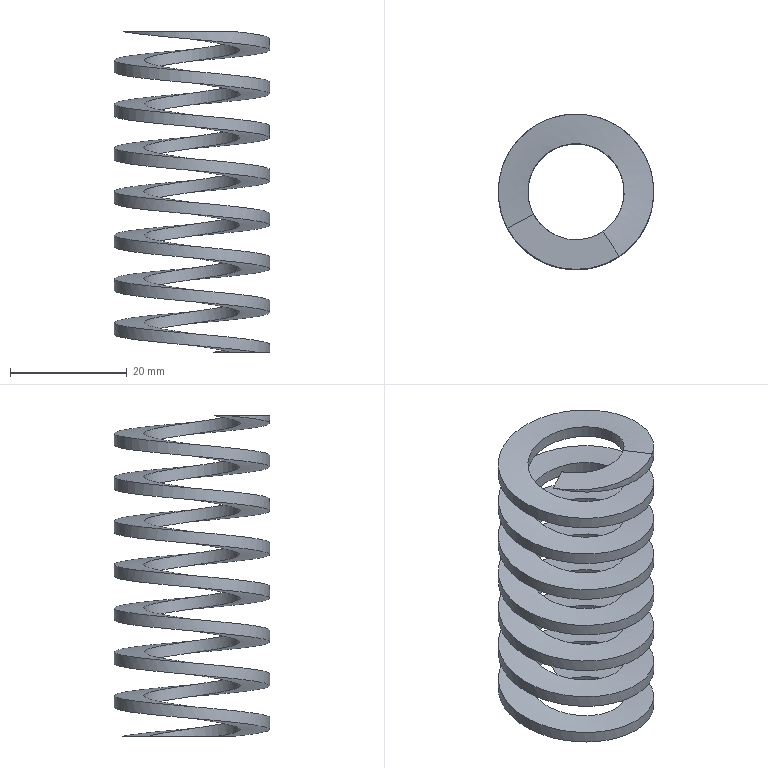Part | STEP file | SWY24.5-55_Default | 1 solid | 6 faces | box 26.648 x 26.648 x 55 mm | volume 5041 mm3 | spline 4 | plane 2